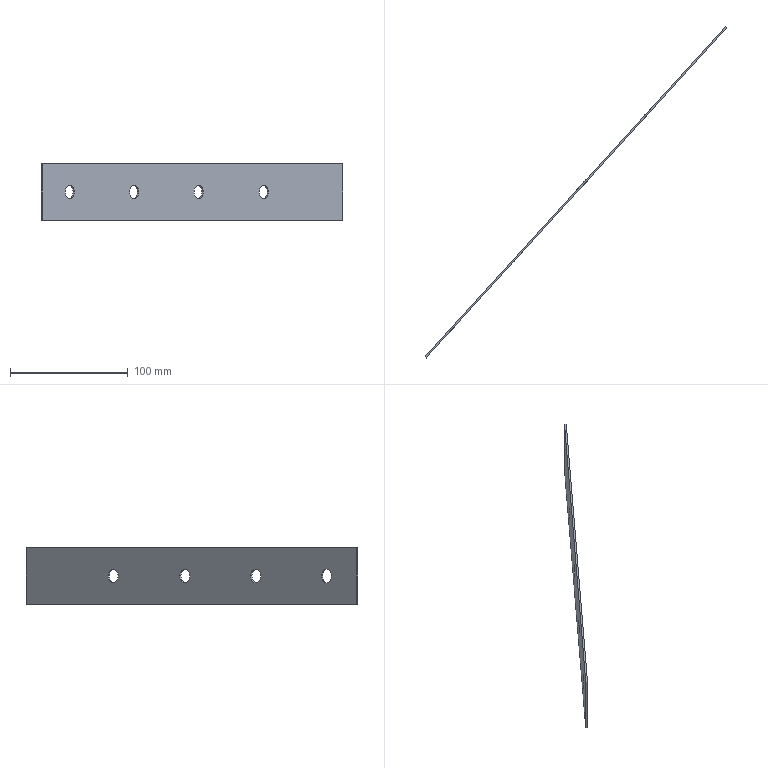Part | STEP file | PRT0001_68_28 | 1 solid | 14 faces | box 256.776 x 282.202 x 48 mm | volume 26740 mm3 | cylinder 8 | plane 6 | commonest cylinder face diameters 11.5 x8
STEP:
#1=CARTESIAN_POINT('',(0.,0.,0.));
#2=DIRECTION('',(0.,0.,1.));
#3=DIRECTION('',(1.,0.,0.));
#4=AXIS2_PLACEMENT_3D('',#1,#2,#3);
#5=CARTESIAN_POINT('',(1942.954,1036.757,0.000000606));
#6=VERTEX_POINT('',#5);
#7=CARTESIAN_POINT('',(1950.69,1045.266,0.000000606));
#8=VERTEX_POINT('',#7);
#9=CARTESIAN_POINT('',(1946.822,1041.012,0.000000606));
#10=DIRECTION('',(0.7399,-0.6727,0.));
#11=DIRECTION('',(-0.6727,-0.7399,0.));
#12=AXIS2_PLACEMENT_3D('',#9,#10,#11);
#13=CIRCLE('',#12,5.75);
#14=CARTESIAN_POINT('',(1897.745,1085.634,0.000000606));
#15=DIRECTION('',(0.7399,-0.6727,0.));
#16=DIRECTION('',(0.6727,0.7399,0.));
#17=AXIS2_PLACEMENT_3D('',#14,#15,#16);
#18=CYLINDRICAL_SURFACE('',#17,5.75);
#19=CARTESIAN_POINT('',(3.142,66.33));
#20=DIRECTION('',(1.,0.));
#21=VECTOR('',#20,1.);
#22=LINE('',#19,#21);
#23=(GEOMETRIC_REPRESENTATION_CONTEXT(2)PARAMETRIC_REPRESENTATION_CONTEXT()REPRESENTATION_CONTEXT('',''));
#24=DEFINITIONAL_REPRESENTATION('',(#22),#23);
#25=PCURVE('',#18,#24);
#26=CARTESIAN_POINT('',(1758.411,833.789,-24.));
#27=DIRECTION('',(0.7399,-0.6727,0.));
#28=DIRECTION('',(0.6727,0.7399,0.));
#29=AXIS2_PLACEMENT_3D('',#26,#27,#28);
#30=PLANE('',#29);
#31=CARTESIAN_POINT('',(280.071,24.));
#32=DIRECTION('',(-1.,0.));
#33=AXIS2_PLACEMENT_2D('',#31,#32);
#34=CIRCLE('',#33,5.75);
#35=(GEOMETRIC_REPRESENTATION_CONTEXT(2)PARAMETRIC_REPRESENTATION_CONTEXT()REPRESENTATION_CONTEXT('',''));
#36=DEFINITIONAL_REPRESENTATION('',(#34),#35);
#37=PCURVE('',#30,#36);
#38=SURFACE_CURVE('',#13,(#25,#37),.PCURVE_S1.);
#39=EDGE_CURVE('',#6,#8,#38,.T.);
#40=ORIENTED_EDGE('',*,*,#39,.F.);
#41=CARTESIAN_POINT('',(1941.844,1037.767,0.000000606));
#42=VERTEX_POINT('',#41);
#43=CARTESIAN_POINT('',(1942.954,1036.757,0.000000606));
#44=DIRECTION('',(-0.7399,0.6727,0.));
#45=VECTOR('',#44,1.);
#46=LINE('',#43,#45);
#47=CARTESIAN_POINT('',(3.142,66.33));
#48=DIRECTION('',(0.,-1.));
#49=VECTOR('',#48,1.);
#50=LINE('',#47,#49);
#51=(GEOMETRIC_REPRESENTATION_CONTEXT(2)PARAMETRIC_REPRESENTATION_CONTEXT()REPRESENTATION_CONTEXT('',''));
#52=DEFINITIONAL_REPRESENTATION('',(#50),#51);
#53=PCURVE('',#18,#52);
#54=CARTESIAN_POINT('',(1897.745,1085.634,0.000000606));
#55=DIRECTION('',(0.7399,-0.6727,0.));
#56=DIRECTION('',(0.6727,0.7399,0.));
#57=AXIS2_PLACEMENT_3D('',#54,#55,#56);
#58=CYLINDRICAL_SURFACE('',#57,5.75);
#59=CARTESIAN_POINT('',(3.142,66.33));
#60=DIRECTION('',(0.,-1.));
#61=VECTOR('',#60,1.);
#62=LINE('',#59,#61);
#63=(GEOMETRIC_REPRESENTATION_CONTEXT(2)PARAMETRIC_REPRESENTATION_CONTEXT()REPRESENTATION_CONTEXT('',''));
#64=DEFINITIONAL_REPRESENTATION('',(#62),#63);
#65=PCURVE('',#58,#64);
#66=SURFACE_CURVE('',#46,(#53,#65),.PCURVE_S1.);
#67=EDGE_CURVE('',#6,#42,#66,.T.);
#68=ORIENTED_EDGE('',*,*,#67,.T.);
#69=CARTESIAN_POINT('',(1949.58,1046.275,0.000000606));
#70=VERTEX_POINT('',#69);
#71=CARTESIAN_POINT('',(1945.712,1042.021,0.000000606));
#72=DIRECTION('',(-0.7399,0.6727,0.));
#73=DIRECTION('',(0.6727,0.7399,0.));
#74=AXIS2_PLACEMENT_3D('',#71,#72,#73);
#75=CIRCLE('',#74,5.75);
#76=CARTESIAN_POINT('',(6.283,64.83));
#77=DIRECTION('',(-1.,0.));
#78=VECTOR('',#77,1.);
#79=LINE('',#76,#78);
#80=(GEOMETRIC_REPRESENTATION_CONTEXT(2)PARAMETRIC_REPRESENTATION_CONTEXT()REPRESENTATION_CONTEXT('',''));
#81=DEFINITIONAL_REPRESENTATION('',(#79),#80);
#82=PCURVE('',#18,#81);
#83=CARTESIAN_POINT('',(2012.967,1115.991,-24.));
#84=DIRECTION('',(-0.7399,0.6727,0.));
#85=DIRECTION('',(-0.6727,-0.7399,0.));
#86=AXIS2_PLACEMENT_3D('',#83,#84,#85);
#87=PLANE('',#86);
#88=CARTESIAN_POINT('',(99.975,24.));
#89=DIRECTION('',(-1.,0.));
#90=AXIS2_PLACEMENT_2D('',#88,#89);
#91=CIRCLE('',#90,5.75);
#92=(GEOMETRIC_REPRESENTATION_CONTEXT(2)PARAMETRIC_REPRESENTATION_CONTEXT()REPRESENTATION_CONTEXT('',''));
#93=DEFINITIONAL_REPRESENTATION('',(#91),#92);
#94=PCURVE('',#87,#93);
#95=SURFACE_CURVE('',#75,(#82,#94),.PCURVE_S1.);
#96=EDGE_CURVE('',#70,#42,#95,.T.);
#97=ORIENTED_EDGE('',*,*,#96,.F.);
#98=CARTESIAN_POINT('',(1950.69,1045.266,0.000000606));
#99=DIRECTION('',(-0.7399,0.6727,0.));
#100=VECTOR('',#99,1.);
#101=LINE('',#98,#100);
#102=CARTESIAN_POINT('',(6.283,66.33));
#103=DIRECTION('',(0.,-1.));
#104=VECTOR('',#103,1.);
#105=LINE('',#102,#104);
#106=(GEOMETRIC_REPRESENTATION_CONTEXT(2)PARAMETRIC_REPRESENTATION_CONTEXT()REPRESENTATION_CONTEXT('',''));
#107=DEFINITIONAL_REPRESENTATION('',(#105),#106);
#108=PCURVE('',#18,#107);
#109=CARTESIAN_POINT('',(0.,66.33));
#110=DIRECTION('',(0.,-1.));
#111=VECTOR('',#110,1.);
#112=LINE('',#109,#111);
#113=(GEOMETRIC_REPRESENTATION_CONTEXT(2)PARAMETRIC_REPRESENTATION_CONTEXT()REPRESENTATION_CONTEXT('',''));
#114=DEFINITIONAL_REPRESENTATION('',(#112),#113);
#115=PCURVE('',#58,#114);
#116=SURFACE_CURVE('',#101,(#108,#115),.PCURVE_S1.);
#117=EDGE_CURVE('',#8,#70,#116,.T.);
#118=ORIENTED_EDGE('',*,*,#117,.F.);
#119=EDGE_LOOP('',(#40,#68,#97,#118));
#120=FACE_BOUND('',#119,.F.);
#121=ADVANCED_FACE('',(#120),#18,.F.);
#122=CARTESIAN_POINT('',(1758.411,833.789,-24.));
#123=VERTEX_POINT('',#122);
#124=CARTESIAN_POINT('',(2014.077,1114.982,-24.));
#125=VERTEX_POINT('',#124);
#126=CARTESIAN_POINT('',(1758.411,833.789,-24.));
#127=DIRECTION('',(0.6727,0.7399,0.));
#128=VECTOR('',#127,1.);
#129=LINE('',#126,#128);
#130=CARTESIAN_POINT('',(0.,0.));
#131=DIRECTION('',(1.,0.));
#132=VECTOR('',#131,1.);
#133=LINE('',#130,#132);
#134=(GEOMETRIC_REPRESENTATION_CONTEXT(2)PARAMETRIC_REPRESENTATION_CONTEXT()REPRESENTATION_CONTEXT('',''));
#135=DEFINITIONAL_REPRESENTATION('',(#133),#134);
#136=PCURVE('',#30,#135);
#137=CARTESIAN_POINT('',(0.,0.,-24.));
#138=DIRECTION('',(0.,0.,1.));
#139=DIRECTION('',(1.,0.,0.));
#140=AXIS2_PLACEMENT_3D('',#137,#138,#139);
#141=PLANE('',#140);
#142=CARTESIAN_POINT('',(1758.411,833.789));
#143=DIRECTION('',(0.6727,0.7399));
#144=VECTOR('',#143,1.);
#145=LINE('',#142,#144);
#146=(GEOMETRIC_REPRESENTATION_CONTEXT(2)PARAMETRIC_REPRESENTATION_CONTEXT()REPRESENTATION_CONTEXT('',''));
#147=DEFINITIONAL_REPRESENTATION('',(#145),#146);
#148=PCURVE('',#141,#147);
#149=SURFACE_CURVE('',#129,(#136,#148),.PCURVE_S1.);
#150=EDGE_CURVE('',#123,#125,#149,.T.);
#151=ORIENTED_EDGE('',*,*,#150,.F.);
#152=CARTESIAN_POINT('',(1758.411,833.789,24.));
#153=VERTEX_POINT('',#152);
#154=CARTESIAN_POINT('',(1758.411,833.789,24.));
#155=DIRECTION('',(0.,0.,-1.));
#156=VECTOR('',#155,1.);
#157=LINE('',#154,#156);
#158=CARTESIAN_POINT('',(0.,48.));
#159=DIRECTION('',(0.,-1.));
#160=VECTOR('',#159,1.);
#161=LINE('',#158,#160);
#162=(GEOMETRIC_REPRESENTATION_CONTEXT(2)PARAMETRIC_REPRESENTATION_CONTEXT()REPRESENTATION_CONTEXT('',''));
#163=DEFINITIONAL_REPRESENTATION('',(#161),#162);
#164=PCURVE('',#30,#163);
#165=CARTESIAN_POINT('',(1757.301,834.798,-24.));
#166=DIRECTION('',(-0.6727,-0.7399,0.));
#167=DIRECTION('',(0.7399,-0.6727,0.));
#168=AXIS2_PLACEMENT_3D('',#165,#166,#167);
#169=PLANE('',#168);
#170=CARTESIAN_POINT('',(1.5,48.));
#171=DIRECTION('',(0.,-1.));
#172=VECTOR('',#171,1.);
#173=LINE('',#170,#172);
#174=(GEOMETRIC_REPRESENTATION_CONTEXT(2)PARAMETRIC_REPRESENTATION_CONTEXT()REPRESENTATION_CONTEXT('',''));
#175=DEFINITIONAL_REPRESENTATION('',(#173),#174);
#176=PCURVE('',#169,#175);
#177=SURFACE_CURVE('',#157,(#164,#176),.PCURVE_S1.);
#178=EDGE_CURVE('',#153,#123,#177,.T.);
#179=ORIENTED_EDGE('',*,*,#178,.F.);
#180=CARTESIAN_POINT('',(2014.077,1114.982,24.));
#181=VERTEX_POINT('',#180);
#182=CARTESIAN_POINT('',(2014.077,1114.982,24.));
#183=DIRECTION('',(-0.6727,-0.7399,0.));
#184=VECTOR('',#183,1.);
#185=LINE('',#182,#184);
#186=CARTESIAN_POINT('',(380.046,48.));
#187=DIRECTION('',(-1.,0.));
#188=VECTOR('',#187,1.);
#189=LINE('',#186,#188);
#190=(GEOMETRIC_REPRESENTATION_CONTEXT(2)PARAMETRIC_REPRESENTATION_CONTEXT()REPRESENTATION_CONTEXT('',''));
#191=DEFINITIONAL_REPRESENTATION('',(#189),#190);
#192=PCURVE('',#30,#191);
#193=CARTESIAN_POINT('',(0.,0.,24.));
#194=DIRECTION('',(0.,0.,1.));
#195=DIRECTION('',(1.,0.,0.));
#196=AXIS2_PLACEMENT_3D('',#193,#194,#195);
#197=PLANE('',#196);
#198=CARTESIAN_POINT('',(2014.077,1114.982));
#199=DIRECTION('',(-0.6727,-0.7399));
#200=VECTOR('',#199,1.);
#201=LINE('',#198,#200);
#202=(GEOMETRIC_REPRESENTATION_CONTEXT(2)PARAMETRIC_REPRESENTATION_CONTEXT()REPRESENTATION_CONTEXT('',''));
#203=DEFINITIONAL_REPRESENTATION('',(#201),#202);
#204=PCURVE('',#197,#203);
#205=SURFACE_CURVE('',#185,(#192,#204),.PCURVE_S1.);
#206=EDGE_CURVE('',#181,#153,#205,.T.);
#207=ORIENTED_EDGE('',*,*,#206,.F.);
#208=CARTESIAN_POINT('',(2014.077,1114.982,24.));
#209=DIRECTION('',(0.,0.,-1.));
#210=VECTOR('',#209,1.);
#211=LINE('',#208,#210);
#212=CARTESIAN_POINT('',(380.046,48.));
#213=DIRECTION('',(0.,-1.));
#214=VECTOR('',#213,1.);
#215=LINE('',#212,#214);
#216=(GEOMETRIC_REPRESENTATION_CONTEXT(2)PARAMETRIC_REPRESENTATION_CONTEXT()REPRESENTATION_CONTEXT('',''));
#217=DEFINITIONAL_REPRESENTATION('',(#215),#216);
#218=PCURVE('',#30,#217);
#219=CARTESIAN_POINT('',(2014.077,1114.982,-24.));
#220=DIRECTION('',(0.6727,0.7399,0.));
#221=DIRECTION('',(-0.7399,0.6727,0.));
#222=AXIS2_PLACEMENT_3D('',#219,#220,#221);
#223=PLANE('',#222);
#224=CARTESIAN_POINT('',(0.000000217,48.));
#225=DIRECTION('',(0.,-1.));
#226=VECTOR('',#225,1.);
#227=LINE('',#224,#226);
#228=(GEOMETRIC_REPRESENTATION_CONTEXT(2)PARAMETRIC_REPRESENTATION_CONTEXT()REPRESENTATION_CONTEXT('',''));
#229=DEFINITIONAL_REPRESENTATION('',(#227),#228);
#230=PCURVE('',#223,#229);
#231=SURFACE_CURVE('',#211,(#218,#230),.PCURVE_S1.);
#232=EDGE_CURVE('',#181,#125,#231,.T.);
#233=ORIENTED_EDGE('',*,*,#232,.T.);
#234=EDGE_LOOP('',(#151,#179,#207,#233));
#235=FACE_BOUND('',#234,.F.);
#236=CARTESIAN_POINT('',(1785.651,863.749,0.000000606));
#237=VERTEX_POINT('',#236);
#238=CARTESIAN_POINT('',(1777.914,855.24,0.000000606));
#239=VERTEX_POINT('',#238);
#240=CARTESIAN_POINT('',(1781.782,859.494,0.000000606));
#241=DIRECTION('',(0.7399,-0.6727,0.));
#242=DIRECTION('',(0.6727,0.7399,0.));
#243=AXIS2_PLACEMENT_3D('',#240,#241,#242);
#244=CIRCLE('',#243,5.75);
#245=CARTESIAN_POINT('',(34.742,24.));
#246=DIRECTION('',(1.,0.));
#247=AXIS2_PLACEMENT_2D('',#245,#246);
#248=CIRCLE('',#247,5.75);
#249=(GEOMETRIC_REPRESENTATION_CONTEXT(2)PARAMETRIC_REPRESENTATION_CONTEXT()REPRESENTATION_CONTEXT('',''));
#250=DEFINITIONAL_REPRESENTATION('',(#248),#249);
#251=PCURVE('',#30,#250);
#252=CARTESIAN_POINT('',(1732.705,904.116,0.000000606));
#253=DIRECTION('',(0.7399,-0.6727,0.));
#254=DIRECTION('',(0.6727,0.7399,0.));
#255=AXIS2_PLACEMENT_3D('',#252,#253,#254);
#256=CYLINDRICAL_SURFACE('',#255,5.75);
#257=CARTESIAN_POINT('',(0.,66.33));
#258=DIRECTION('',(1.,0.));
#259=VECTOR('',#258,1.);
#260=LINE('',#257,#259);
#261=(GEOMETRIC_REPRESENTATION_CONTEXT(2)PARAMETRIC_REPRESENTATION_CONTEXT()REPRESENTATION_CONTEXT('',''));
#262=DEFINITIONAL_REPRESENTATION('',(#260),#261);
#263=PCURVE('',#256,#262);
#264=SURFACE_CURVE('',#244,(#251,#263),.PCURVE_S1.);
#265=EDGE_CURVE('',#237,#239,#264,.T.);
#266=ORIENTED_EDGE('',*,*,#265,.T.);
#267=CARTESIAN_POINT('',(1781.782,859.494,0.000000606));
#268=DIRECTION('',(0.7399,-0.6727,0.));
#269=DIRECTION('',(-0.6727,-0.7399,0.));
#270=AXIS2_PLACEMENT_3D('',#267,#268,#269);
#271=CIRCLE('',#270,5.75);
#272=CARTESIAN_POINT('',(34.742,24.));
#273=DIRECTION('',(-1.,0.));
#274=AXIS2_PLACEMENT_2D('',#272,#273);
#275=CIRCLE('',#274,5.75);
#276=(GEOMETRIC_REPRESENTATION_CONTEXT(2)PARAMETRIC_REPRESENTATION_CONTEXT()REPRESENTATION_CONTEXT('',''));
#277=DEFINITIONAL_REPRESENTATION('',(#275),#276);
#278=PCURVE('',#30,#277);
#279=CARTESIAN_POINT('',(1732.705,904.116,0.000000606));
#280=DIRECTION('',(0.7399,-0.6727,0.));
#281=DIRECTION('',(0.6727,0.7399,0.));
#282=AXIS2_PLACEMENT_3D('',#279,#280,#281);
#283=CYLINDRICAL_SURFACE('',#282,5.75);
#284=CARTESIAN_POINT('',(3.142,66.33));
#285=DIRECTION('',(1.,0.));
#286=VECTOR('',#285,1.);
#287=LINE('',#284,#286);
#288=(GEOMETRIC_REPRESENTATION_CONTEXT(2)PARAMETRIC_REPRESENTATION_CONTEXT()REPRESENTATION_CONTEXT('',''));
#289=DEFINITIONAL_REPRESENTATION('',(#287),#288);
#290=PCURVE('',#283,#289);
#291=SURFACE_CURVE('',#271,(#278,#290),.PCURVE_S1.);
#292=EDGE_CURVE('',#239,#237,#291,.T.);
#293=ORIENTED_EDGE('',*,*,#292,.T.);
#294=EDGE_LOOP('',(#266,#293));
#295=FACE_BOUND('',#294,.F.);
#296=CARTESIAN_POINT('',(1840.425,923.992,0.000000606));
#297=VERTEX_POINT('',#296);
#298=CARTESIAN_POINT('',(1832.689,915.483,0.000000606));
#299=VERTEX_POINT('',#298);
#300=CARTESIAN_POINT('',(1836.557,919.738,0.000000606));
#301=DIRECTION('',(0.7399,-0.6727,0.));
#302=DIRECTION('',(0.6727,0.7399,0.));
#303=AXIS2_PLACEMENT_3D('',#300,#301,#302);
#304=CIRCLE('',#303,5.75);
#305=CARTESIAN_POINT('',(116.163,24.));
#306=DIRECTION('',(1.,0.));
#307=AXIS2_PLACEMENT_2D('',#305,#306);
#308=CIRCLE('',#307,5.75);
#309=(GEOMETRIC_REPRESENTATION_CONTEXT(2)PARAMETRIC_REPRESENTATION_CONTEXT()REPRESENTATION_CONTEXT('',''));
#310=DEFINITIONAL_REPRESENTATION('',(#308),#309);
#311=PCURVE('',#30,#310);
#312=CARTESIAN_POINT('',(1787.48,964.359,0.000000606));
#313=DIRECTION('',(0.7399,-0.6727,0.));
#314=DIRECTION('',(0.6727,0.7399,0.));
#315=AXIS2_PLACEMENT_3D('',#312,#313,#314);
#316=CYLINDRICAL_SURFACE('',#315,5.75);
#317=CARTESIAN_POINT('',(0.,66.33));
#318=DIRECTION('',(1.,0.));
#319=VECTOR('',#318,1.);
#320=LINE('',#317,#319);
#321=(GEOMETRIC_REPRESENTATION_CONTEXT(2)PARAMETRIC_REPRESENTATION_CONTEXT()REPRESENTATION_CONTEXT('',''));
#322=DEFINITIONAL_REPRESENTATION('',(#320),#321);
#323=PCURVE('',#316,#322);
#324=SURFACE_CURVE('',#304,(#311,#323),.PCURVE_S1.);
#325=EDGE_CURVE('',#297,#299,#324,.T.);
#326=ORIENTED_EDGE('',*,*,#325,.T.);
#327=CARTESIAN_POINT('',(1836.557,919.738,0.000000606));
#328=DIRECTION('',(0.7399,-0.6727,0.));
#329=DIRECTION('',(-0.6727,-0.7399,0.));
#330=AXIS2_PLACEMENT_3D('',#327,#328,#329);
#331=CIRCLE('',#330,5.75);
#332=CARTESIAN_POINT('',(116.163,24.));
#333=DIRECTION('',(-1.,0.));
#334=AXIS2_PLACEMENT_2D('',#332,#333);
#335=CIRCLE('',#334,5.75);
#336=(GEOMETRIC_REPRESENTATION_CONTEXT(2)PARAMETRIC_REPRESENTATION_CONTEXT()REPRESENTATION_CONTEXT('',''));
#337=DEFINITIONAL_REPRESENTATION('',(#335),#336);
#338=PCURVE('',#30,#337);
#339=CARTESIAN_POINT('',(1787.48,964.359,0.000000606));
#340=DIRECTION('',(0.7399,-0.6727,0.));
#341=DIRECTION('',(0.6727,0.7399,0.));
#342=AXIS2_PLACEMENT_3D('',#339,#340,#341);
#343=CYLINDRICAL_SURFACE('',#342,5.75);
#344=CARTESIAN_POINT('',(3.142,66.33));
#345=DIRECTION('',(1.,0.));
#346=VECTOR('',#345,1.);
#347=LINE('',#344,#346);
#348=(GEOMETRIC_REPRESENTATION_CONTEXT(2)PARAMETRIC_REPRESENTATION_CONTEXT()REPRESENTATION_CONTEXT('',''));
#349=DEFINITIONAL_REPRESENTATION('',(#347),#348);
#350=PCURVE('',#343,#349);
#351=SURFACE_CURVE('',#331,(#338,#350),.PCURVE_S1.);
#352=EDGE_CURVE('',#299,#297,#351,.T.);
#353=ORIENTED_EDGE('',*,*,#352,.T.);
#354=EDGE_LOOP('',(#326,#353));
#355=FACE_BOUND('',#354,.F.);
#356=CARTESIAN_POINT('',(1895.221,984.259,0.000000606));
#357=VERTEX_POINT('',#356);
#358=CARTESIAN_POINT('',(1887.485,975.751,0.000000606));
#359=VERTEX_POINT('',#358);
#360=CARTESIAN_POINT('',(1891.353,980.005,0.000000606));
#361=DIRECTION('',(0.7399,-0.6727,0.));
#362=DIRECTION('',(0.6727,0.7399,0.));
#363=AXIS2_PLACEMENT_3D('',#360,#361,#362);
#364=CIRCLE('',#363,5.75);
#365=CARTESIAN_POINT('',(197.618,24.));
#366=DIRECTION('',(1.,0.));
#367=AXIS2_PLACEMENT_2D('',#365,#366);
#368=CIRCLE('',#367,5.75);
#369=(GEOMETRIC_REPRESENTATION_CONTEXT(2)PARAMETRIC_REPRESENTATION_CONTEXT()REPRESENTATION_CONTEXT('',''));
#370=DEFINITIONAL_REPRESENTATION('',(#368),#369);
#371=PCURVE('',#30,#370);
#372=CARTESIAN_POINT('',(1842.276,1024.627,0.000000606));
#373=DIRECTION('',(0.7399,-0.6727,0.));
#374=DIRECTION('',(0.6727,0.7399,0.));
#375=AXIS2_PLACEMENT_3D('',#372,#373,#374);
#376=CYLINDRICAL_SURFACE('',#375,5.75);
#377=CARTESIAN_POINT('',(0.,66.33));
#378=DIRECTION('',(1.,0.));
#379=VECTOR('',#378,1.);
#380=LINE('',#377,#379);
#381=(GEOMETRIC_REPRESENTATION_CONTEXT(2)PARAMETRIC_REPRESENTATION_CONTEXT()REPRESENTATION_CONTEXT('',''));
#382=DEFINITIONAL_REPRESENTATION('',(#380),#381);
#383=PCURVE('',#376,#382);
#384=SURFACE_CURVE('',#364,(#371,#383),.PCURVE_S1.);
#385=EDGE_CURVE('',#357,#359,#384,.T.);
#386=ORIENTED_EDGE('',*,*,#385,.T.);
#387=CARTESIAN_POINT('',(1891.353,980.005,0.000000606));
#388=DIRECTION('',(0.7399,-0.6727,0.));
#389=DIRECTION('',(-0.6727,-0.7399,0.));
#390=AXIS2_PLACEMENT_3D('',#387,#388,#389);
#391=CIRCLE('',#390,5.75);
#392=CARTESIAN_POINT('',(197.618,24.));
#393=DIRECTION('',(-1.,0.));
#394=AXIS2_PLACEMENT_2D('',#392,#393);
#395=CIRCLE('',#394,5.75);
#396=(GEOMETRIC_REPRESENTATION_CONTEXT(2)PARAMETRIC_REPRESENTATION_CONTEXT()REPRESENTATION_CONTEXT('',''));
#397=DEFINITIONAL_REPRESENTATION('',(#395),#396);
#398=PCURVE('',#30,#397);
#399=CARTESIAN_POINT('',(1842.276,1024.627,0.000000606));
#400=DIRECTION('',(0.7399,-0.6727,0.));
#401=DIRECTION('',(0.6727,0.7399,0.));
#402=AXIS2_PLACEMENT_3D('',#399,#400,#401);
#403=CYLINDRICAL_SURFACE('',#402,5.75);
#404=CARTESIAN_POINT('',(3.142,66.33));
#405=DIRECTION('',(1.,0.));
#406=VECTOR('',#405,1.);
#407=LINE('',#404,#406);
#408=(GEOMETRIC_REPRESENTATION_CONTEXT(2)PARAMETRIC_REPRESENTATION_CONTEXT()REPRESENTATION_CONTEXT('',''));
#409=DEFINITIONAL_REPRESENTATION('',(#407),#408);
#410=PCURVE('',#403,#409);
#411=SURFACE_CURVE('',#391,(#398,#410),.PCURVE_S1.);
#412=EDGE_CURVE('',#359,#357,#411,.T.);
#413=ORIENTED_EDGE('',*,*,#412,.T.);
#414=EDGE_LOOP('',(#386,#413));
#415=FACE_BOUND('',#414,.F.);
#416=CARTESIAN_POINT('',(1946.822,1041.012,0.000000606));
#417=DIRECTION('',(0.7399,-0.6727,0.));
#418=DIRECTION('',(0.6727,0.7399,0.));
#419=AXIS2_PLACEMENT_3D('',#416,#417,#418);
#420=CIRCLE('',#419,5.75);
#421=CARTESIAN_POINT('',(280.071,24.));
#422=DIRECTION('',(1.,0.));
#423=AXIS2_PLACEMENT_2D('',#421,#422);
#424=CIRCLE('',#423,5.75);
#425=(GEOMETRIC_REPRESENTATION_CONTEXT(2)PARAMETRIC_REPRESENTATION_CONTEXT()REPRESENTATION_CONTEXT('',''));
#426=DEFINITIONAL_REPRESENTATION('',(#424),#425);
#427=PCURVE('',#30,#426);
#428=CARTESIAN_POINT('',(0.,66.33));
#429=DIRECTION('',(1.,0.));
#430=VECTOR('',#429,1.);
#431=LINE('',#428,#430);
#432=(GEOMETRIC_REPRESENTATION_CONTEXT(2)PARAMETRIC_REPRESENTATION_CONTEXT()REPRESENTATION_CONTEXT('',''));
#433=DEFINITIONAL_REPRESENTATION('',(#431),#432);
#434=PCURVE('',#58,#433);
#435=SURFACE_CURVE('',#420,(#427,#434),.PCURVE_S1.);
#436=EDGE_CURVE('',#8,#6,#435,.T.);
#437=ORIENTED_EDGE('',*,*,#436,.T.);
#438=ORIENTED_EDGE('',*,*,#39,.T.);
#439=EDGE_LOOP('',(#437,#438));
#440=FACE_BOUND('',#439,.F.);
#441=ADVANCED_FACE('',(#235,#295,#355,#415,#440),#30,.T.);
#442=CARTESIAN_POINT('',(1757.301,834.798,-24.));
#443=VERTEX_POINT('',#442);
#444=CARTESIAN_POINT('',(1757.301,834.798,-24.));
#445=DIRECTION('',(0.7399,-0.6727,0.));
#446=VECTOR('',#445,1.);
#447=LINE('',#444,#446);
#448=CARTESIAN_POINT('',(1757.301,834.798));
#449=DIRECTION('',(0.7399,-0.6727));
#450=VECTOR('',#449,1.);
#451=LINE('',#448,#450);
#452=(GEOMETRIC_REPRESENTATION_CONTEXT(2)PARAMETRIC_REPRESENTATION_CONTEXT()REPRESENTATION_CONTEXT('',''));
#453=DEFINITIONAL_REPRESENTATION('',(#451),#452);
#454=PCURVE('',#141,#453);
#455=CARTESIAN_POINT('',(0.,0.));
#456=DIRECTION('',(1.,0.));
#457=VECTOR('',#456,1.);
#458=LINE('',#455,#457);
#459=(GEOMETRIC_REPRESENTATION_CONTEXT(2)PARAMETRIC_REPRESENTATION_CONTEXT()REPRESENTATION_CONTEXT('',''));
#460=DEFINITIONAL_REPRESENTATION('',(#458),#459);
#461=PCURVE('',#169,#460);
#462=SURFACE_CURVE('',#447,(#454,#461),.PCURVE_S1.);
#463=EDGE_CURVE('',#443,#123,#462,.T.);
#464=ORIENTED_EDGE('',*,*,#463,.T.);
#465=ORIENTED_EDGE('',*,*,#150,.T.);
#466=CARTESIAN_POINT('',(2012.967,1115.991,-24.));
#467=VERTEX_POINT('',#466);
#468=CARTESIAN_POINT('',(2014.077,1114.982,-24.));
#469=DIRECTION('',(-0.7399,0.6727,0.));
#470=VECTOR('',#469,1.);
#471=LINE('',#468,#470);
#472=CARTESIAN_POINT('',(2014.077,1114.982));
#473=DIRECTION('',(-0.7399,0.6727));
#474=VECTOR('',#473,1.);
#475=LINE('',#472,#474);
#476=(GEOMETRIC_REPRESENTATION_CONTEXT(2)PARAMETRIC_REPRESENTATION_CONTEXT()REPRESENTATION_CONTEXT('',''));
#477=DEFINITIONAL_REPRESENTATION('',(#475),#476);
#478=PCURVE('',#141,#477);
#479=CARTESIAN_POINT('',(0.000000217,0.));
#480=DIRECTION('',(1.,0.));
#481=VECTOR('',#480,1.);
#482=LINE('',#479,#481);
#483=(GEOMETRIC_REPRESENTATION_CONTEXT(2)PARAMETRIC_REPRESENTATION_CONTEXT()REPRESENTATION_CONTEXT('',''));
#484=DEFINITIONAL_REPRESENTATION('',(#482),#483);
#485=PCURVE('',#223,#484);
#486=SURFACE_CURVE('',#471,(#478,#485),.PCURVE_S1.);
#487=EDGE_CURVE('',#125,#467,#486,.T.);
#488=ORIENTED_EDGE('',*,*,#487,.T.);
#489=CARTESIAN_POINT('',(2012.967,1115.991,-24.));
#490=DIRECTION('',(-0.6727,-0.7399,0.));
#491=VECTOR('',#490,1.);
#492=LINE('',#489,#491);
#493=CARTESIAN_POINT('',(2012.967,1115.991));
#494=DIRECTION('',(-0.6727,-0.7399));
#495=VECTOR('',#494,1.);
#496=LINE('',#493,#495);
#497=(GEOMETRIC_REPRESENTATION_CONTEXT(2)PARAMETRIC_REPRESENTATION_CONTEXT()REPRESENTATION_CONTEXT('',''));
#498=DEFINITIONAL_REPRESENTATION('',(#496),#497);
#499=PCURVE('',#141,#498);
#500=CARTESIAN_POINT('',(-0.00001299,0.));
#501=DIRECTION('',(1.,0.));
#502=VECTOR('',#501,1.);
#503=LINE('',#500,#502);
#504=(GEOMETRIC_REPRESENTATION_CONTEXT(2)PARAMETRIC_REPRESENTATION_CONTEXT()REPRESENTATION_CONTEXT('',''));
#505=DEFINITIONAL_REPRESENTATION('',(#503),#504);
#506=PCURVE('',#87,#505);
#507=SURFACE_CURVE('',#492,(#499,#506),.PCURVE_S1.);
#508=EDGE_CURVE('',#467,#443,#507,.T.);
#509=ORIENTED_EDGE('',*,*,#508,.T.);
#510=EDGE_LOOP('',(#464,#465,#488,#509));
#511=FACE_BOUND('',#510,.F.);
#512=ADVANCED_FACE('',(#511),#141,.F.);
#513=ORIENTED_EDGE('',*,*,#463,.F.);
#514=CARTESIAN_POINT('',(1757.301,834.798,24.));
#515=VERTEX_POINT('',#514);
#516=CARTESIAN_POINT('',(1757.301,834.798,24.));
#517=DIRECTION('',(0.,0.,-1.));
#518=VECTOR('',#517,1.);
#519=LINE('',#516,#518);
#520=CARTESIAN_POINT('',(0.,48.));
#521=DIRECTION('',(0.,-1.));
#522=VECTOR('',#521,1.);
#523=LINE('',#520,#522);
#524=(GEOMETRIC_REPRESENTATION_CONTEXT(2)PARAMETRIC_REPRESENTATION_CONTEXT()REPRESENTATION_CONTEXT('',''));
#525=DEFINITIONAL_REPRESENTATION('',(#523),#524);
#526=PCURVE('',#169,#525);
#527=CARTESIAN_POINT('',(380.046,48.));
#528=DIRECTION('',(0.,-1.));
#529=VECTOR('',#528,1.);
#530=LINE('',#527,#529);
#531=(GEOMETRIC_REPRESENTATION_CONTEXT(2)PARAMETRIC_REPRESENTATION_CONTEXT()REPRESENTATION_CONTEXT('',''));
#532=DEFINITIONAL_REPRESENTATION('',(#530),#531);
#533=PCURVE('',#87,#532);
#534=SURFACE_CURVE('',#519,(#526,#533),.PCURVE_S1.);
#535=EDGE_CURVE('',#515,#443,#534,.T.);
#536=ORIENTED_EDGE('',*,*,#535,.F.);
#537=CARTESIAN_POINT('',(1758.411,833.789,24.));
#538=DIRECTION('',(-0.7399,0.6727,0.));
#539=VECTOR('',#538,1.);
#540=LINE('',#537,#539);
#541=CARTESIAN_POINT('',(1.5,48.));
#542=DIRECTION('',(-1.,0.));
#543=VECTOR('',#542,1.);
#544=LINE('',#541,#543);
#545=(GEOMETRIC_REPRESENTATION_CONTEXT(2)PARAMETRIC_REPRESENTATION_CONTEXT()REPRESENTATION_CONTEXT('',''));
#546=DEFINITIONAL_REPRESENTATION('',(#544),#545);
#547=PCURVE('',#169,#546);
#548=CARTESIAN_POINT('',(1758.411,833.789));
#549=DIRECTION('',(-0.7399,0.6727));
#550=VECTOR('',#549,1.);
#551=LINE('',#548,#550);
#552=(GEOMETRIC_REPRESENTATION_CONTEXT(2)PARAMETRIC_REPRESENTATION_CONTEXT()REPRESENTATION_CONTEXT('',''));
#553=DEFINITIONAL_REPRESENTATION('',(#551),#552);
#554=PCURVE('',#197,#553);
#555=SURFACE_CURVE('',#540,(#547,#554),.PCURVE_S1.);
#556=EDGE_CURVE('',#153,#515,#555,.T.);
#557=ORIENTED_EDGE('',*,*,#556,.F.);
#558=ORIENTED_EDGE('',*,*,#178,.T.);
#559=EDGE_LOOP('',(#513,#536,#557,#558));
#560=FACE_BOUND('',#559,.F.);
#561=ADVANCED_FACE('',(#560),#169,.T.);
#562=ORIENTED_EDGE('',*,*,#508,.F.);
#563=CARTESIAN_POINT('',(2012.967,1115.991,24.));
#564=VERTEX_POINT('',#563);
#565=CARTESIAN_POINT('',(2012.967,1115.991,24.));
#566=DIRECTION('',(0.,0.,-1.));
#567=VECTOR('',#566,1.);
#568=LINE('',#565,#567);
#569=CARTESIAN_POINT('',(-0.00001299,48.));
#570=DIRECTION('',(0.,-1.));
#571=VECTOR('',#570,1.);
#572=LINE('',#569,#571);
#573=(GEOMETRIC_REPRESENTATION_CONTEXT(2)PARAMETRIC_REPRESENTATION_CONTEXT()REPRESENTATION_CONTEXT('',''));
#574=DEFINITIONAL_REPRESENTATION('',(#572),#573);
#575=PCURVE('',#87,#574);
#576=CARTESIAN_POINT('',(1.5,48.));
#577=DIRECTION('',(0.,-1.));
#578=VECTOR('',#577,1.);
#579=LINE('',#576,#578);
#580=(GEOMETRIC_REPRESENTATION_CONTEXT(2)PARAMETRIC_REPRESENTATION_CONTEXT()REPRESENTATION_CONTEXT('',''));
#581=DEFINITIONAL_REPRESENTATION('',(#579),#580);
#582=PCURVE('',#223,#581);
#583=SURFACE_CURVE('',#568,(#575,#582),.PCURVE_S1.);
#584=EDGE_CURVE('',#564,#467,#583,.T.);
#585=ORIENTED_EDGE('',*,*,#584,.F.);
#586=CARTESIAN_POINT('',(1757.301,834.798,24.));
#587=DIRECTION('',(0.6727,0.7399,0.));
#588=VECTOR('',#587,1.);
#589=LINE('',#586,#588);
#590=CARTESIAN_POINT('',(380.046,48.));
#591=DIRECTION('',(-1.,0.));
#592=VECTOR('',#591,1.);
#593=LINE('',#590,#592);
#594=(GEOMETRIC_REPRESENTATION_CONTEXT(2)PARAMETRIC_REPRESENTATION_CONTEXT()REPRESENTATION_CONTEXT('',''));
#595=DEFINITIONAL_REPRESENTATION('',(#593),#594);
#596=PCURVE('',#87,#595);
#597=CARTESIAN_POINT('',(1757.301,834.798));
#598=DIRECTION('',(0.6727,0.7399));
#599=VECTOR('',#598,1.);
#600=LINE('',#597,#599);
#601=(GEOMETRIC_REPRESENTATION_CONTEXT(2)PARAMETRIC_REPRESENTATION_CONTEXT()REPRESENTATION_CONTEXT('',''));
#602=DEFINITIONAL_REPRESENTATION('',(#600),#601);
#603=PCURVE('',#197,#602);
#604=SURFACE_CURVE('',#589,(#596,#603),.PCURVE_S1.);
#605=EDGE_CURVE('',#515,#564,#604,.T.);
#606=ORIENTED_EDGE('',*,*,#605,.F.);
#607=ORIENTED_EDGE('',*,*,#535,.T.);
#608=EDGE_LOOP('',(#562,#585,#606,#607));
#609=FACE_BOUND('',#608,.F.);
#610=CARTESIAN_POINT('',(1776.804,856.249,0.000000606));
#611=VERTEX_POINT('',#610);
#612=CARTESIAN_POINT('',(1784.541,864.758,0.000000606));
#613=VERTEX_POINT('',#612);
#614=CARTESIAN_POINT('',(1780.673,860.504,0.000000606));
#615=DIRECTION('',(-0.7399,0.6727,0.));
#616=DIRECTION('',(-0.6727,-0.7399,0.));
#617=AXIS2_PLACEMENT_3D('',#614,#615,#616);
#618=CIRCLE('',#617,5.75);
#619=CARTESIAN_POINT('',(345.304,24.));
#620=DIRECTION('',(1.,0.));
#621=AXIS2_PLACEMENT_2D('',#619,#620);
#622=CIRCLE('',#621,5.75);
#623=(GEOMETRIC_REPRESENTATION_CONTEXT(2)PARAMETRIC_REPRESENTATION_CONTEXT()REPRESENTATION_CONTEXT('',''));
#624=DEFINITIONAL_REPRESENTATION('',(#622),#623);
#625=PCURVE('',#87,#624);
#626=CARTESIAN_POINT('',(3.142,64.83));
#627=DIRECTION('',(-1.,0.));
#628=VECTOR('',#627,1.);
#629=LINE('',#626,#628);
#630=(GEOMETRIC_REPRESENTATION_CONTEXT(2)PARAMETRIC_REPRESENTATION_CONTEXT()REPRESENTATION_CONTEXT('',''));
#631=DEFINITIONAL_REPRESENTATION('',(#629),#630);
#632=PCURVE('',#256,#631);
#633=SURFACE_CURVE('',#618,(#625,#632),.PCURVE_S1.);
#634=EDGE_CURVE('',#611,#613,#633,.T.);
#635=ORIENTED_EDGE('',*,*,#634,.T.);
#636=CARTESIAN_POINT('',(1780.673,860.504,0.000000606));
#637=DIRECTION('',(-0.7399,0.6727,0.));
#638=DIRECTION('',(0.6727,0.7399,0.));
#639=AXIS2_PLACEMENT_3D('',#636,#637,#638);
#640=CIRCLE('',#639,5.75);
#641=CARTESIAN_POINT('',(345.304,24.));
#642=DIRECTION('',(-1.,0.));
#643=AXIS2_PLACEMENT_2D('',#641,#642);
#644=CIRCLE('',#643,5.75);
#645=(GEOMETRIC_REPRESENTATION_CONTEXT(2)PARAMETRIC_REPRESENTATION_CONTEXT()REPRESENTATION_CONTEXT('',''));
#646=DEFINITIONAL_REPRESENTATION('',(#644),#645);
#647=PCURVE('',#87,#646);
#648=CARTESIAN_POINT('',(6.283,64.83));
#649=DIRECTION('',(-1.,0.));
#650=VECTOR('',#649,1.);
#651=LINE('',#648,#650);
#652=(GEOMETRIC_REPRESENTATION_CONTEXT(2)PARAMETRIC_REPRESENTATION_CONTEXT()REPRESENTATION_CONTEXT('',''));
#653=DEFINITIONAL_REPRESENTATION('',(#651),#652);
#654=PCURVE('',#283,#653);
#655=SURFACE_CURVE('',#640,(#647,#654),.PCURVE_S1.);
#656=EDGE_CURVE('',#613,#611,#655,.T.);
#657=ORIENTED_EDGE('',*,*,#656,.T.);
#658=EDGE_LOOP('',(#635,#657));
#659=FACE_BOUND('',#658,.F.);
#660=CARTESIAN_POINT('',(1831.579,916.492,0.000000606));
#661=VERTEX_POINT('',#660);
#662=CARTESIAN_POINT('',(1839.315,925.001,0.000000606));
#663=VERTEX_POINT('',#662);
#664=CARTESIAN_POINT('',(1835.447,920.747,0.000000606));
#665=DIRECTION('',(-0.7399,0.6727,0.));
#666=DIRECTION('',(-0.6727,-0.7399,0.));
#667=AXIS2_PLACEMENT_3D('',#664,#665,#666);
#668=CIRCLE('',#667,5.75);
#669=CARTESIAN_POINT('',(263.883,24.));
#670=DIRECTION('',(1.,0.));
#671=AXIS2_PLACEMENT_2D('',#669,#670);
#672=CIRCLE('',#671,5.75);
#673=(GEOMETRIC_REPRESENTATION_CONTEXT(2)PARAMETRIC_REPRESENTATION_CONTEXT()REPRESENTATION_CONTEXT('',''));
#674=DEFINITIONAL_REPRESENTATION('',(#672),#673);
#675=PCURVE('',#87,#674);
#676=CARTESIAN_POINT('',(3.142,64.83));
#677=DIRECTION('',(-1.,0.));
#678=VECTOR('',#677,1.);
#679=LINE('',#676,#678);
#680=(GEOMETRIC_REPRESENTATION_CONTEXT(2)PARAMETRIC_REPRESENTATION_CONTEXT()REPRESENTATION_CONTEXT('',''));
#681=DEFINITIONAL_REPRESENTATION('',(#679),#680);
#682=PCURVE('',#316,#681);
#683=SURFACE_CURVE('',#668,(#675,#682),.PCURVE_S1.);
#684=EDGE_CURVE('',#661,#663,#683,.T.);
#685=ORIENTED_EDGE('',*,*,#684,.T.);
#686=CARTESIAN_POINT('',(1835.447,920.747,0.000000606));
#687=DIRECTION('',(-0.7399,0.6727,0.));
#688=DIRECTION('',(0.6727,0.7399,0.));
#689=AXIS2_PLACEMENT_3D('',#686,#687,#688);
#690=CIRCLE('',#689,5.75);
#691=CARTESIAN_POINT('',(263.883,24.));
#692=DIRECTION('',(-1.,0.));
#693=AXIS2_PLACEMENT_2D('',#691,#692);
#694=CIRCLE('',#693,5.75);
#695=(GEOMETRIC_REPRESENTATION_CONTEXT(2)PARAMETRIC_REPRESENTATION_CONTEXT()REPRESENTATION_CONTEXT('',''));
#696=DEFINITIONAL_REPRESENTATION('',(#694),#695);
#697=PCURVE('',#87,#696);
#698=CARTESIAN_POINT('',(6.283,64.83));
#699=DIRECTION('',(-1.,0.));
#700=VECTOR('',#699,1.);
#701=LINE('',#698,#700);
#702=(GEOMETRIC_REPRESENTATION_CONTEXT(2)PARAMETRIC_REPRESENTATION_CONTEXT()REPRESENTATION_CONTEXT('',''));
#703=DEFINITIONAL_REPRESENTATION('',(#701),#702);
#704=PCURVE('',#343,#703);
#705=SURFACE_CURVE('',#690,(#697,#704),.PCURVE_S1.);
#706=EDGE_CURVE('',#663,#661,#705,.T.);
#707=ORIENTED_EDGE('',*,*,#706,.T.);
#708=EDGE_LOOP('',(#685,#707));
#709=FACE_BOUND('',#708,.F.);
#710=CARTESIAN_POINT('',(1886.375,976.76,0.000000606));
#711=VERTEX_POINT('',#710);
#712=CARTESIAN_POINT('',(1894.111,985.268,0.000000606));
#713=VERTEX_POINT('',#712);
#714=CARTESIAN_POINT('',(1890.243,981.014,0.000000606));
#715=DIRECTION('',(-0.7399,0.6727,0.));
#716=DIRECTION('',(-0.6727,-0.7399,0.));
#717=AXIS2_PLACEMENT_3D('',#714,#715,#716);
#718=CIRCLE('',#717,5.75);
#719=CARTESIAN_POINT('',(182.428,24.));
#720=DIRECTION('',(1.,0.));
#721=AXIS2_PLACEMENT_2D('',#719,#720);
#722=CIRCLE('',#721,5.75);
#723=(GEOMETRIC_REPRESENTATION_CONTEXT(2)PARAMETRIC_REPRESENTATION_CONTEXT()REPRESENTATION_CONTEXT('',''));
#724=DEFINITIONAL_REPRESENTATION('',(#722),#723);
#725=PCURVE('',#87,#724);
#726=CARTESIAN_POINT('',(3.142,64.83));
#727=DIRECTION('',(-1.,0.));
#728=VECTOR('',#727,1.);
#729=LINE('',#726,#728);
#730=(GEOMETRIC_REPRESENTATION_CONTEXT(2)PARAMETRIC_REPRESENTATION_CONTEXT()REPRESENTATION_CONTEXT('',''));
#731=DEFINITIONAL_REPRESENTATION('',(#729),#730);
#732=PCURVE('',#376,#731);
#733=SURFACE_CURVE('',#718,(#725,#732),.PCURVE_S1.);
#734=EDGE_CURVE('',#711,#713,#733,.T.);
#735=ORIENTED_EDGE('',*,*,#734,.T.);
#736=CARTESIAN_POINT('',(1890.243,981.014,0.000000606));
#737=DIRECTION('',(-0.7399,0.6727,0.));
#738=DIRECTION('',(0.6727,0.7399,0.));
#739=AXIS2_PLACEMENT_3D('',#736,#737,#738);
#740=CIRCLE('',#739,5.75);
#741=CARTESIAN_POINT('',(182.428,24.));
#742=DIRECTION('',(-1.,0.));
#743=AXIS2_PLACEMENT_2D('',#741,#742);
#744=CIRCLE('',#743,5.75);
#745=(GEOMETRIC_REPRESENTATION_CONTEXT(2)PARAMETRIC_REPRESENTATION_CONTEXT()REPRESENTATION_CONTEXT('',''));
#746=DEFINITIONAL_REPRESENTATION('',(#744),#745);
#747=PCURVE('',#87,#746);
#748=CARTESIAN_POINT('',(6.283,64.83));
#749=DIRECTION('',(-1.,0.));
#750=VECTOR('',#749,1.);
#751=LINE('',#748,#750);
#752=(GEOMETRIC_REPRESENTATION_CONTEXT(2)PARAMETRIC_REPRESENTATION_CONTEXT()REPRESENTATION_CONTEXT('',''));
#753=DEFINITIONAL_REPRESENTATION('',(#751),#752);
#754=PCURVE('',#403,#753);
#755=SURFACE_CURVE('',#740,(#747,#754),.PCURVE_S1.);
#756=EDGE_CURVE('',#713,#711,#755,.T.);
#757=ORIENTED_EDGE('',*,*,#756,.T.);
#758=EDGE_LOOP('',(#735,#757));
#759=FACE_BOUND('',#758,.F.);
#760=CARTESIAN_POINT('',(1945.712,1042.021,0.000000606));
#761=DIRECTION('',(-0.7399,0.6727,0.));
#762=DIRECTION('',(-0.6727,-0.7399,0.));
#763=AXIS2_PLACEMENT_3D('',#760,#761,#762);
#764=CIRCLE('',#763,5.75);
#765=CARTESIAN_POINT('',(99.975,24.));
#766=DIRECTION('',(1.,0.));
#767=AXIS2_PLACEMENT_2D('',#765,#766);
#768=CIRCLE('',#767,5.75);
#769=(GEOMETRIC_REPRESENTATION_CONTEXT(2)PARAMETRIC_REPRESENTATION_CONTEXT()REPRESENTATION_CONTEXT('',''));
#770=DEFINITIONAL_REPRESENTATION('',(#768),#769);
#771=PCURVE('',#87,#770);
#772=CARTESIAN_POINT('',(3.142,64.83));
#773=DIRECTION('',(-1.,0.));
#774=VECTOR('',#773,1.);
#775=LINE('',#772,#774);
#776=(GEOMETRIC_REPRESENTATION_CONTEXT(2)PARAMETRIC_REPRESENTATION_CONTEXT()REPRESENTATION_CONTEXT('',''));
#777=DEFINITIONAL_REPRESENTATION('',(#775),#776);
#778=PCURVE('',#58,#777);
#779=SURFACE_CURVE('',#764,(#771,#778),.PCURVE_S1.);
#780=EDGE_CURVE('',#42,#70,#779,.T.);
#781=ORIENTED_EDGE('',*,*,#780,.T.);
#782=ORIENTED_EDGE('',*,*,#96,.T.);
#783=EDGE_LOOP('',(#781,#782));
#784=FACE_BOUND('',#783,.F.);
#785=ADVANCED_FACE('',(#609,#659,#709,#759,#784),#87,.T.);
#786=ORIENTED_EDGE('',*,*,#584,.F.);
#787=CARTESIAN_POINT('',(2012.967,1115.991,24.));
#788=DIRECTION('',(0.7399,-0.6727,0.));
#789=VECTOR('',#788,1.);
#790=LINE('',#787,#789);
#791=CARTESIAN_POINT('',(1.5,48.));
#792=DIRECTION('',(-1.,0.));
#793=VECTOR('',#792,1.);
#794=LINE('',#791,#793);
#795=(GEOMETRIC_REPRESENTATION_CONTEXT(2)PARAMETRIC_REPRESENTATION_CONTEXT()REPRESENTATION_CONTEXT('',''));
#796=DEFINITIONAL_REPRESENTATION('',(#794),#795);
#797=PCURVE('',#223,#796);
#798=CARTESIAN_POINT('',(2012.967,1115.991));
#799=DIRECTION('',(0.7399,-0.6727));
#800=VECTOR('',#799,1.);
#801=LINE('',#798,#800);
#802=(GEOMETRIC_REPRESENTATION_CONTEXT(2)PARAMETRIC_REPRESENTATION_CONTEXT()REPRESENTATION_CONTEXT('',''));
#803=DEFINITIONAL_REPRESENTATION('',(#801),#802);
#804=PCURVE('',#197,#803);
#805=SURFACE_CURVE('',#790,(#797,#804),.PCURVE_S1.);
#806=EDGE_CURVE('',#564,#181,#805,.T.);
#807=ORIENTED_EDGE('',*,*,#806,.T.);
#808=ORIENTED_EDGE('',*,*,#232,.T.);
#809=ORIENTED_EDGE('',*,*,#487,.T.);
#810=EDGE_LOOP('',(#786,#807,#808,#809));
#811=FACE_BOUND('',#810,.T.);
#812=ADVANCED_FACE('',(#811),#223,.T.);
#813=ORIENTED_EDGE('',*,*,#556,.T.);
#814=ORIENTED_EDGE('',*,*,#605,.T.);
#815=ORIENTED_EDGE('',*,*,#806,.T.);
#816=ORIENTED_EDGE('',*,*,#206,.T.);
#817=EDGE_LOOP('',(#813,#814,#815,#816));
#818=FACE_BOUND('',#817,.F.);
#819=ADVANCED_FACE('',(#818),#197,.T.);
#820=ORIENTED_EDGE('',*,*,#265,.F.);
#821=CARTESIAN_POINT('',(1785.651,863.749,0.000000606));
#822=DIRECTION('',(-0.7399,0.6727,0.));
#823=VECTOR('',#822,1.);
#824=LINE('',#821,#823);
#825=CARTESIAN_POINT('',(0.,66.33));
#826=DIRECTION('',(0.,-1.));
#827=VECTOR('',#826,1.);
#828=LINE('',#825,#827);
#829=(GEOMETRIC_REPRESENTATION_CONTEXT(2)PARAMETRIC_REPRESENTATION_CONTEXT()REPRESENTATION_CONTEXT('',''));
#830=DEFINITIONAL_REPRESENTATION('',(#828),#829);
#831=PCURVE('',#256,#830);
#832=CARTESIAN_POINT('',(6.283,66.33));
#833=DIRECTION('',(0.,-1.));
#834=VECTOR('',#833,1.);
#835=LINE('',#832,#834);
#836=(GEOMETRIC_REPRESENTATION_CONTEXT(2)PARAMETRIC_REPRESENTATION_CONTEXT()REPRESENTATION_CONTEXT('',''));
#837=DEFINITIONAL_REPRESENTATION('',(#835),#836);
#838=PCURVE('',#283,#837);
#839=SURFACE_CURVE('',#824,(#831,#838),.PCURVE_S1.);
#840=EDGE_CURVE('',#237,#613,#839,.T.);
#841=ORIENTED_EDGE('',*,*,#840,.T.);
#842=ORIENTED_EDGE('',*,*,#634,.F.);
#843=CARTESIAN_POINT('',(1777.914,855.24,0.000000606));
#844=DIRECTION('',(-0.7399,0.6727,0.));
#845=VECTOR('',#844,1.);
#846=LINE('',#843,#845);
#847=CARTESIAN_POINT('',(3.142,66.33));
#848=DIRECTION('',(0.,-1.));
#849=VECTOR('',#848,1.);
#850=LINE('',#847,#849);
#851=(GEOMETRIC_REPRESENTATION_CONTEXT(2)PARAMETRIC_REPRESENTATION_CONTEXT()REPRESENTATION_CONTEXT('',''));
#852=DEFINITIONAL_REPRESENTATION('',(#850),#851);
#853=PCURVE('',#256,#852);
#854=CARTESIAN_POINT('',(3.142,66.33));
#855=DIRECTION('',(0.,-1.));
#856=VECTOR('',#855,1.);
#857=LINE('',#854,#856);
#858=(GEOMETRIC_REPRESENTATION_CONTEXT(2)PARAMETRIC_REPRESENTATION_CONTEXT()REPRESENTATION_CONTEXT('',''));
#859=DEFINITIONAL_REPRESENTATION('',(#857),#858);
#860=PCURVE('',#283,#859);
#861=SURFACE_CURVE('',#846,(#853,#860),.PCURVE_S1.);
#862=EDGE_CURVE('',#239,#611,#861,.T.);
#863=ORIENTED_EDGE('',*,*,#862,.F.);
#864=EDGE_LOOP('',(#820,#841,#842,#863));
#865=FACE_BOUND('',#864,.F.);
#866=ADVANCED_FACE('',(#865),#256,.F.);
#867=ORIENTED_EDGE('',*,*,#292,.F.);
#868=ORIENTED_EDGE('',*,*,#862,.T.);
#869=ORIENTED_EDGE('',*,*,#656,.F.);
#870=ORIENTED_EDGE('',*,*,#840,.F.);
#871=EDGE_LOOP('',(#867,#868,#869,#870));
#872=FACE_BOUND('',#871,.F.);
#873=ADVANCED_FACE('',(#872),#283,.F.);
#874=ORIENTED_EDGE('',*,*,#325,.F.);
#875=CARTESIAN_POINT('',(1840.425,923.992,0.000000606));
#876=DIRECTION('',(-0.7399,0.6727,0.));
#877=VECTOR('',#876,1.);
#878=LINE('',#875,#877);
#879=CARTESIAN_POINT('',(0.,66.33));
#880=DIRECTION('',(0.,-1.));
#881=VECTOR('',#880,1.);
#882=LINE('',#879,#881);
#883=(GEOMETRIC_REPRESENTATION_CONTEXT(2)PARAMETRIC_REPRESENTATION_CONTEXT()REPRESENTATION_CONTEXT('',''));
#884=DEFINITIONAL_REPRESENTATION('',(#882),#883);
#885=PCURVE('',#316,#884);
#886=CARTESIAN_POINT('',(6.283,66.33));
#887=DIRECTION('',(0.,-1.));
#888=VECTOR('',#887,1.);
#889=LINE('',#886,#888);
#890=(GEOMETRIC_REPRESENTATION_CONTEXT(2)PARAMETRIC_REPRESENTATION_CONTEXT()REPRESENTATION_CONTEXT('',''));
#891=DEFINITIONAL_REPRESENTATION('',(#889),#890);
#892=PCURVE('',#343,#891);
#893=SURFACE_CURVE('',#878,(#885,#892),.PCURVE_S1.);
#894=EDGE_CURVE('',#297,#663,#893,.T.);
#895=ORIENTED_EDGE('',*,*,#894,.T.);
#896=ORIENTED_EDGE('',*,*,#684,.F.);
#897=CARTESIAN_POINT('',(1832.689,915.483,0.000000606));
#898=DIRECTION('',(-0.7399,0.6727,0.));
#899=VECTOR('',#898,1.);
#900=LINE('',#897,#899);
#901=CARTESIAN_POINT('',(3.142,66.33));
#902=DIRECTION('',(0.,-1.));
#903=VECTOR('',#902,1.);
#904=LINE('',#901,#903);
#905=(GEOMETRIC_REPRESENTATION_CONTEXT(2)PARAMETRIC_REPRESENTATION_CONTEXT()REPRESENTATION_CONTEXT('',''));
#906=DEFINITIONAL_REPRESENTATION('',(#904),#905);
#907=PCURVE('',#316,#906);
#908=CARTESIAN_POINT('',(3.142,66.33));
#909=DIRECTION('',(0.,-1.));
#910=VECTOR('',#909,1.);
#911=LINE('',#908,#910);
#912=(GEOMETRIC_REPRESENTATION_CONTEXT(2)PARAMETRIC_REPRESENTATION_CONTEXT()REPRESENTATION_CONTEXT('',''));
#913=DEFINITIONAL_REPRESENTATION('',(#911),#912);
#914=PCURVE('',#343,#913);
#915=SURFACE_CURVE('',#900,(#907,#914),.PCURVE_S1.);
#916=EDGE_CURVE('',#299,#661,#915,.T.);
#917=ORIENTED_EDGE('',*,*,#916,.F.);
#918=EDGE_LOOP('',(#874,#895,#896,#917));
#919=FACE_BOUND('',#918,.F.);
#920=ADVANCED_FACE('',(#919),#316,.F.);
#921=ORIENTED_EDGE('',*,*,#352,.F.);
#922=ORIENTED_EDGE('',*,*,#916,.T.);
#923=ORIENTED_EDGE('',*,*,#706,.F.);
#924=ORIENTED_EDGE('',*,*,#894,.F.);
#925=EDGE_LOOP('',(#921,#922,#923,#924));
#926=FACE_BOUND('',#925,.F.);
#927=ADVANCED_FACE('',(#926),#343,.F.);
#928=ORIENTED_EDGE('',*,*,#385,.F.);
#929=CARTESIAN_POINT('',(1895.221,984.259,0.000000606));
#930=DIRECTION('',(-0.7399,0.6727,0.));
#931=VECTOR('',#930,1.);
#932=LINE('',#929,#931);
#933=CARTESIAN_POINT('',(0.,66.33));
#934=DIRECTION('',(0.,-1.));
#935=VECTOR('',#934,1.);
#936=LINE('',#933,#935);
#937=(GEOMETRIC_REPRESENTATION_CONTEXT(2)PARAMETRIC_REPRESENTATION_CONTEXT()REPRESENTATION_CONTEXT('',''));
#938=DEFINITIONAL_REPRESENTATION('',(#936),#937);
#939=PCURVE('',#376,#938);
#940=CARTESIAN_POINT('',(6.283,66.33));
#941=DIRECTION('',(0.,-1.));
#942=VECTOR('',#941,1.);
#943=LINE('',#940,#942);
#944=(GEOMETRIC_REPRESENTATION_CONTEXT(2)PARAMETRIC_REPRESENTATION_CONTEXT()REPRESENTATION_CONTEXT('',''));
#945=DEFINITIONAL_REPRESENTATION('',(#943),#944);
#946=PCURVE('',#403,#945);
#947=SURFACE_CURVE('',#932,(#939,#946),.PCURVE_S1.);
#948=EDGE_CURVE('',#357,#713,#947,.T.);
#949=ORIENTED_EDGE('',*,*,#948,.T.);
#950=ORIENTED_EDGE('',*,*,#734,.F.);
#951=CARTESIAN_POINT('',(1887.485,975.751,0.000000606));
#952=DIRECTION('',(-0.7399,0.6727,0.));
#953=VECTOR('',#952,1.);
#954=LINE('',#951,#953);
#955=CARTESIAN_POINT('',(3.142,66.33));
#956=DIRECTION('',(0.,-1.));
#957=VECTOR('',#956,1.);
#958=LINE('',#955,#957);
#959=(GEOMETRIC_REPRESENTATION_CONTEXT(2)PARAMETRIC_REPRESENTATION_CONTEXT()REPRESENTATION_CONTEXT('',''));
#960=DEFINITIONAL_REPRESENTATION('',(#958),#959);
#961=PCURVE('',#376,#960);
#962=CARTESIAN_POINT('',(3.142,66.33));
#963=DIRECTION('',(0.,-1.));
#964=VECTOR('',#963,1.);
#965=LINE('',#962,#964);
#966=(GEOMETRIC_REPRESENTATION_CONTEXT(2)PARAMETRIC_REPRESENTATION_CONTEXT()REPRESENTATION_CONTEXT('',''));
#967=DEFINITIONAL_REPRESENTATION('',(#965),#966);
#968=PCURVE('',#403,#967);
#969=SURFACE_CURVE('',#954,(#961,#968),.PCURVE_S1.);
#970=EDGE_CURVE('',#359,#711,#969,.T.);
#971=ORIENTED_EDGE('',*,*,#970,.F.);
#972=EDGE_LOOP('',(#928,#949,#950,#971));
#973=FACE_BOUND('',#972,.F.);
#974=ADVANCED_FACE('',(#973),#376,.F.);
#975=ORIENTED_EDGE('',*,*,#412,.F.);
#976=ORIENTED_EDGE('',*,*,#970,.T.);
#977=ORIENTED_EDGE('',*,*,#756,.F.);
#978=ORIENTED_EDGE('',*,*,#948,.F.);
#979=EDGE_LOOP('',(#975,#976,#977,#978));
#980=FACE_BOUND('',#979,.F.);
#981=ADVANCED_FACE('',(#980),#403,.F.);
#982=ORIENTED_EDGE('',*,*,#436,.F.);
#983=ORIENTED_EDGE('',*,*,#117,.T.);
#984=ORIENTED_EDGE('',*,*,#780,.F.);
#985=ORIENTED_EDGE('',*,*,#67,.F.);
#986=EDGE_LOOP('',(#982,#983,#984,#985));
#987=FACE_BOUND('',#986,.F.);
#988=ADVANCED_FACE('',(#987),#58,.F.);
#989=CLOSED_SHELL('',(#121,#441,#512,#561,#785,#812,#819,#866,#873,#920,#927,#974,#981,#988));
#990=MANIFOLD_SOLID_BREP('',#989);
#991=(LENGTH_UNIT()NAMED_UNIT(*)SI_UNIT(.MILLI.,.METRE.));
#992=UNCERTAINTY_MEASURE_WITH_UNIT(LENGTH_MEASURE(0.0000005),#991,'','');
#993=(NAMED_UNIT(*)PLANE_ANGLE_UNIT()SI_UNIT($,.RADIAN.));
#994=(NAMED_UNIT(*)SI_UNIT($,.STERADIAN.)SOLID_ANGLE_UNIT());
#995=(GEOMETRIC_REPRESENTATION_CONTEXT(3)GLOBAL_UNCERTAINTY_ASSIGNED_CONTEXT((#992))GLOBAL_UNIT_ASSIGNED_CONTEXT((#991,#993,#994))REPRESENTATION_CONTEXT('',''));
#996=ADVANCED_BREP_SHAPE_REPRESENTATION('',(#4,#990),#995);